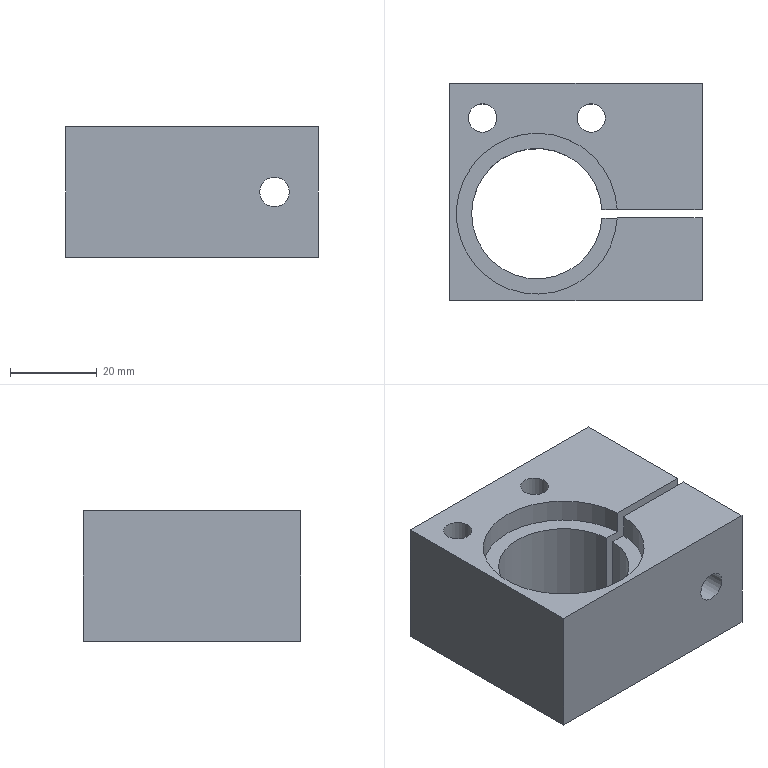Part | STEP file | 1 solid | 22 faces | box 58 x 50 x 30 mm | volume 56140 mm3 | plane 13 | cylinder 9 | commonest cylinder face diameters 6.5 x2 11 x2 6.8 x1 8.5 x1 14 x1 30 x1